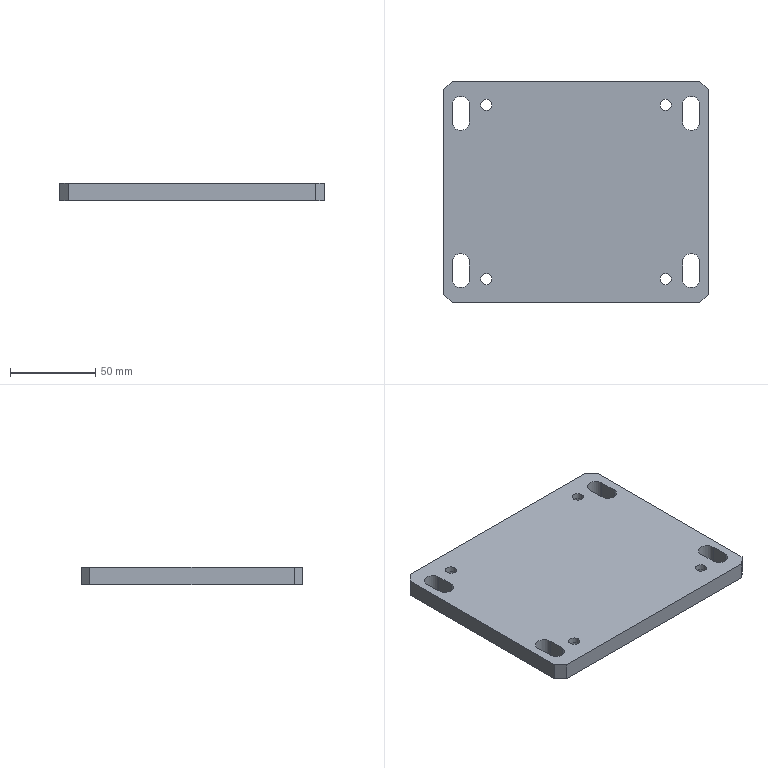Part | NX | 1 solid | 38 faces | box 155 x 130 x 10 mm | volume 190923 mm3 | plane 22 | cylinder 16 | commonest cylinder face diameters 10 x8 6.5 x4 11 x4
STEP:
#1=CARTESIAN_POINT('',(335.5,-45.,-18.));
#2=VERTEX_POINT('',#1);
#3=CARTESIAN_POINT('',(330.5,-40.,-18.));
#4=VERTEX_POINT('',#3);
#5=CARTESIAN_POINT('',(225.067,65.433,-18.));
#6=DIRECTION('',(-0.7071,0.7071,0.));
#7=VECTOR('',#6,1000.);
#8=LINE('',#5,#7);
#9=EDGE_CURVE('',#2,#4,#8,.T.);
#10=ORIENTED_EDGE('',*,*,#9,.F.);
#11=CARTESIAN_POINT('',(335.5,-45.,-28.));
#12=VERTEX_POINT('',#11);
#13=CARTESIAN_POINT('',(335.5,-45.,8.781));
#14=DIRECTION('',(0.,0.,1.));
#15=VECTOR('',#14,1000.);
#16=LINE('',#13,#15);
#17=EDGE_CURVE('',#12,#2,#16,.T.);
#18=ORIENTED_EDGE('',*,*,#17,.F.);
#19=CARTESIAN_POINT('',(330.5,-40.,-28.));
#20=VERTEX_POINT('',#19);
#21=CARTESIAN_POINT('',(407.933,-117.433,-28.));
#22=DIRECTION('',(0.7071,-0.7071,0.));
#23=VECTOR('',#22,1000.);
#24=LINE('',#21,#23);
#25=EDGE_CURVE('',#20,#12,#24,.T.);
#26=ORIENTED_EDGE('',*,*,#25,.F.);
#27=CARTESIAN_POINT('',(330.5,-40.,8.781));
#28=DIRECTION('',(0.,0.,-1.));
#29=VECTOR('',#28,1000.);
#30=LINE('',#27,#29);
#31=EDGE_CURVE('',#4,#20,#30,.T.);
#32=ORIENTED_EDGE('',*,*,#31,.F.);
#33=EDGE_LOOP('',(#10,#18,#26,#32));
#34=FACE_BOUND('',#33,.T.);
#35=CARTESIAN_POINT('',(335.5,-45.,8.781));
#36=DIRECTION('',(-0.7071,-0.7071,0.));
#37=DIRECTION('',(0.,0.,-1.));
#38=AXIS2_PLACEMENT_3D('',#35,#36,#37);
#39=PLANE('',#38);
#40=ADVANCED_FACE('',(#34),#39,.F.);
#41=CARTESIAN_POINT('',(316.,-156.,-28.));
#42=VERTEX_POINT('',#41);
#43=CARTESIAN_POINT('',(310.5,-156.,-28.));
#44=DIRECTION('',(0.,0.,1.));
#45=DIRECTION('',(1.,0.,0.));
#46=AXIS2_PLACEMENT_3D('',#43,#44,#45);
#47=CIRCLE('',#46,5.5);
#48=EDGE_CURVE('',#42,#42,#47,.T.);
#49=ORIENTED_EDGE('',*,*,#48,.F.);
#50=EDGE_LOOP('',(#49));
#51=FACE_BOUND('',#50,.T.);
#52=CARTESIAN_POINT('',(305.,-156.,-21.5));
#53=VERTEX_POINT('',#52);
#54=CARTESIAN_POINT('',(310.5,-156.,-21.5));
#55=DIRECTION('',(0.,0.,1.));
#56=DIRECTION('',(-1.,0.,0.));
#57=AXIS2_PLACEMENT_3D('',#54,#55,#56);
#58=CIRCLE('',#57,5.5);
#59=EDGE_CURVE('',#53,#53,#58,.T.);
#60=ORIENTED_EDGE('',*,*,#59,.T.);
#61=EDGE_LOOP('',(#60));
#62=FACE_BOUND('',#61,.T.);
#63=CARTESIAN_POINT('',(310.5,-156.,-28.));
#64=DIRECTION('',(0.,0.,1.));
#65=DIRECTION('',(0.,-1.,0.));
#66=AXIS2_PLACEMENT_3D('',#63,#64,#65);
#67=CYLINDRICAL_SURFACE('',#66,5.5);
#68=ADVANCED_FACE('',(#51,#62),#67,.F.);
#69=CARTESIAN_POINT('',(316.,-54.,-28.));
#70=VERTEX_POINT('',#69);
#71=CARTESIAN_POINT('',(310.5,-54.,-28.));
#72=DIRECTION('',(0.,0.,1.));
#73=DIRECTION('',(1.,0.,0.));
#74=AXIS2_PLACEMENT_3D('',#71,#72,#73);
#75=CIRCLE('',#74,5.5);
#76=EDGE_CURVE('',#70,#70,#75,.T.);
#77=ORIENTED_EDGE('',*,*,#76,.F.);
#78=EDGE_LOOP('',(#77));
#79=FACE_BOUND('',#78,.T.);
#80=CARTESIAN_POINT('',(316.,-54.,-21.5));
#81=VERTEX_POINT('',#80);
#82=CARTESIAN_POINT('',(310.5,-54.,-21.5));
#83=DIRECTION('',(0.,0.,1.));
#84=DIRECTION('',(1.,0.,0.));
#85=AXIS2_PLACEMENT_3D('',#82,#83,#84);
#86=CIRCLE('',#85,5.5);
#87=EDGE_CURVE('',#81,#81,#86,.T.);
#88=ORIENTED_EDGE('',*,*,#87,.T.);
#89=EDGE_LOOP('',(#88));
#90=FACE_BOUND('',#89,.T.);
#91=CARTESIAN_POINT('',(310.5,-54.,-28.));
#92=DIRECTION('',(0.,0.,1.));
#93=DIRECTION('',(0.,-1.,0.));
#94=AXIS2_PLACEMENT_3D('',#91,#92,#93);
#95=CYLINDRICAL_SURFACE('',#94,5.5);
#96=ADVANCED_FACE('',(#79,#90),#95,.F.);
#97=CARTESIAN_POINT('',(330.5,-54.,-18.));
#98=VERTEX_POINT('',#97);
#99=CARTESIAN_POINT('',(320.5,-54.,-18.));
#100=VERTEX_POINT('',#99);
#101=CARTESIAN_POINT('',(325.5,-54.,-18.));
#102=DIRECTION('',(0.,0.,1.));
#103=DIRECTION('',(1.,0.,0.));
#104=AXIS2_PLACEMENT_3D('',#101,#102,#103);
#105=CIRCLE('',#104,5.);
#106=EDGE_CURVE('',#98,#100,#105,.T.);
#107=ORIENTED_EDGE('',*,*,#106,.T.);
#108=CARTESIAN_POINT('',(320.5,-54.,-28.));
#109=VERTEX_POINT('',#108);
#110=CARTESIAN_POINT('',(320.5,-54.,-23.));
#111=DIRECTION('',(0.,0.,1.));
#112=VECTOR('',#111,1000.);
#113=LINE('',#110,#112);
#114=EDGE_CURVE('',#109,#100,#113,.T.);
#115=ORIENTED_EDGE('',*,*,#114,.F.);
#116=CARTESIAN_POINT('',(330.5,-54.,-28.));
#117=VERTEX_POINT('',#116);
#118=CARTESIAN_POINT('',(325.5,-54.,-28.));
#119=DIRECTION('',(0.,0.,-1.));
#120=DIRECTION('',(1.,0.,0.));
#121=AXIS2_PLACEMENT_3D('',#118,#119,#120);
#122=CIRCLE('',#121,5.);
#123=EDGE_CURVE('',#109,#117,#122,.T.);
#124=ORIENTED_EDGE('',*,*,#123,.T.);
#125=CARTESIAN_POINT('',(330.5,-54.,-23.));
#126=DIRECTION('',(0.,0.,-1.));
#127=VECTOR('',#126,1000.);
#128=LINE('',#125,#127);
#129=EDGE_CURVE('',#98,#117,#128,.T.);
#130=ORIENTED_EDGE('',*,*,#129,.F.);
#131=EDGE_LOOP('',(#107,#115,#124,#130));
#132=FACE_BOUND('',#131,.T.);
#133=CARTESIAN_POINT('',(325.5,-54.,-6.5));
#134=DIRECTION('',(0.,0.,-1.));
#135=DIRECTION('',(0.,1.,0.));
#136=AXIS2_PLACEMENT_3D('',#133,#134,#135);
#137=CYLINDRICAL_SURFACE('',#136,5.);
#138=ADVANCED_FACE('',(#132),#137,.F.);
#139=CARTESIAN_POINT('',(320.5,-64.,-18.));
#140=VERTEX_POINT('',#139);
#141=CARTESIAN_POINT('',(320.5,105.,-18.));
#142=DIRECTION('',(0.,-1.,0.));
#143=VECTOR('',#142,1000.);
#144=LINE('',#141,#143);
#145=EDGE_CURVE('',#100,#140,#144,.T.);
#146=ORIENTED_EDGE('',*,*,#145,.T.);
#147=CARTESIAN_POINT('',(320.5,-64.,-28.));
#148=VERTEX_POINT('',#147);
#149=CARTESIAN_POINT('',(320.5,-64.,-23.));
#150=DIRECTION('',(0.,0.,-1.));
#151=VECTOR('',#150,1000.);
#152=LINE('',#149,#151);
#153=EDGE_CURVE('',#140,#148,#152,.T.);
#154=ORIENTED_EDGE('',*,*,#153,.T.);
#155=CARTESIAN_POINT('',(320.5,105.,-28.));
#156=DIRECTION('',(0.,1.,0.));
#157=VECTOR('',#156,1000.);
#158=LINE('',#155,#157);
#159=EDGE_CURVE('',#148,#109,#158,.T.);
#160=ORIENTED_EDGE('',*,*,#159,.T.);
#161=ORIENTED_EDGE('',*,*,#114,.T.);
#162=EDGE_LOOP('',(#146,#154,#160,#161));
#163=FACE_BOUND('',#162,.T.);
#164=CARTESIAN_POINT('',(320.5,-53.,-6.5));
#165=DIRECTION('',(-1.,0.,0.));
#166=DIRECTION('',(0.,0.,-1.));
#167=AXIS2_PLACEMENT_3D('',#164,#165,#166);
#168=PLANE('',#167);
#169=ADVANCED_FACE('',(#163),#168,.F.);
#170=CARTESIAN_POINT('',(330.5,-64.,-18.));
#171=VERTEX_POINT('',#170);
#172=CARTESIAN_POINT('',(325.5,-64.,-18.));
#173=DIRECTION('',(0.,0.,1.));
#174=DIRECTION('',(1.,0.,0.));
#175=AXIS2_PLACEMENT_3D('',#172,#173,#174);
#176=CIRCLE('',#175,5.);
#177=EDGE_CURVE('',#140,#171,#176,.T.);
#178=ORIENTED_EDGE('',*,*,#177,.T.);
#179=CARTESIAN_POINT('',(330.5,-64.,-28.));
#180=VERTEX_POINT('',#179);
#181=CARTESIAN_POINT('',(330.5,-64.,-23.));
#182=DIRECTION('',(0.,0.,1.));
#183=VECTOR('',#182,1000.);
#184=LINE('',#181,#183);
#185=EDGE_CURVE('',#180,#171,#184,.T.);
#186=ORIENTED_EDGE('',*,*,#185,.F.);
#187=CARTESIAN_POINT('',(325.5,-64.,-28.));
#188=DIRECTION('',(0.,0.,-1.));
#189=DIRECTION('',(1.,0.,0.));
#190=AXIS2_PLACEMENT_3D('',#187,#188,#189);
#191=CIRCLE('',#190,5.);
#192=EDGE_CURVE('',#180,#148,#191,.T.);
#193=ORIENTED_EDGE('',*,*,#192,.T.);
#194=ORIENTED_EDGE('',*,*,#153,.F.);
#195=EDGE_LOOP('',(#178,#186,#193,#194));
#196=FACE_BOUND('',#195,.T.);
#197=CARTESIAN_POINT('',(325.5,-64.,-6.5));
#198=DIRECTION('',(0.,0.,-1.));
#199=DIRECTION('',(0.,1.,0.));
#200=AXIS2_PLACEMENT_3D('',#197,#198,#199);
#201=CYLINDRICAL_SURFACE('',#200,5.);
#202=ADVANCED_FACE('',(#196),#201,.F.);
#203=CARTESIAN_POINT('',(330.5,105.,-18.));
#204=DIRECTION('',(0.,1.,0.));
#205=VECTOR('',#204,1000.);
#206=LINE('',#203,#205);
#207=EDGE_CURVE('',#171,#98,#206,.T.);
#208=ORIENTED_EDGE('',*,*,#207,.T.);
#209=ORIENTED_EDGE('',*,*,#129,.T.);
#210=CARTESIAN_POINT('',(330.5,105.,-28.));
#211=DIRECTION('',(0.,-1.,0.));
#212=VECTOR('',#211,1000.);
#213=LINE('',#210,#212);
#214=EDGE_CURVE('',#117,#180,#213,.T.);
#215=ORIENTED_EDGE('',*,*,#214,.T.);
#216=ORIENTED_EDGE('',*,*,#185,.T.);
#217=EDGE_LOOP('',(#208,#209,#215,#216));
#218=FACE_BOUND('',#217,.T.);
#219=CARTESIAN_POINT('',(330.5,-53.,-6.5));
#220=DIRECTION('',(1.,0.,0.));
#221=DIRECTION('',(0.,0.,1.));
#222=AXIS2_PLACEMENT_3D('',#219,#220,#221);
#223=PLANE('',#222);
#224=ADVANCED_FACE('',(#218),#223,.F.);
#225=CARTESIAN_POINT('',(320.5,-156.,-18.));
#226=VERTEX_POINT('',#225);
#227=CARTESIAN_POINT('',(330.5,-156.,-18.));
#228=VERTEX_POINT('',#227);
#229=CARTESIAN_POINT('',(325.5,-156.,-18.));
#230=DIRECTION('',(0.,0.,1.));
#231=DIRECTION('',(1.,0.,0.));
#232=AXIS2_PLACEMENT_3D('',#229,#230,#231);
#233=CIRCLE('',#232,5.);
#234=EDGE_CURVE('',#226,#228,#233,.T.);
#235=ORIENTED_EDGE('',*,*,#234,.T.);
#236=CARTESIAN_POINT('',(330.5,-156.,-28.));
#237=VERTEX_POINT('',#236);
#238=CARTESIAN_POINT('',(330.5,-156.,-6.5));
#239=DIRECTION('',(0.,0.,1.));
#240=VECTOR('',#239,1000.);
#241=LINE('',#238,#240);
#242=EDGE_CURVE('',#237,#228,#241,.T.);
#243=ORIENTED_EDGE('',*,*,#242,.F.);
#244=CARTESIAN_POINT('',(320.5,-156.,-28.));
#245=VERTEX_POINT('',#244);
#246=CARTESIAN_POINT('',(325.5,-156.,-28.));
#247=DIRECTION('',(0.,0.,-1.));
#248=DIRECTION('',(1.,0.,0.));
#249=AXIS2_PLACEMENT_3D('',#246,#247,#248);
#250=CIRCLE('',#249,5.);
#251=EDGE_CURVE('',#237,#245,#250,.T.);
#252=ORIENTED_EDGE('',*,*,#251,.T.);
#253=CARTESIAN_POINT('',(320.5,-156.,-6.5));
#254=DIRECTION('',(0.,0.,-1.));
#255=VECTOR('',#254,1000.);
#256=LINE('',#253,#255);
#257=EDGE_CURVE('',#226,#245,#256,.T.);
#258=ORIENTED_EDGE('',*,*,#257,.F.);
#259=EDGE_LOOP('',(#235,#243,#252,#258));
#260=FACE_BOUND('',#259,.T.);
#261=CARTESIAN_POINT('',(325.5,-156.,-6.5));
#262=DIRECTION('',(0.,0.,-1.));
#263=DIRECTION('',(0.,-1.,0.));
#264=AXIS2_PLACEMENT_3D('',#261,#262,#263);
#265=CYLINDRICAL_SURFACE('',#264,5.);
#266=ADVANCED_FACE('',(#260),#265,.F.);
#267=CARTESIAN_POINT('',(330.5,-146.,-18.));
#268=VERTEX_POINT('',#267);
#269=CARTESIAN_POINT('',(330.5,-53.,-18.));
#270=DIRECTION('',(0.,1.,0.));
#271=VECTOR('',#270,1000.);
#272=LINE('',#269,#271);
#273=EDGE_CURVE('',#228,#268,#272,.T.);
#274=ORIENTED_EDGE('',*,*,#273,.T.);
#275=CARTESIAN_POINT('',(330.5,-146.,-28.));
#276=VERTEX_POINT('',#275);
#277=CARTESIAN_POINT('',(330.5,-146.,-6.5));
#278=DIRECTION('',(0.,0.,-1.));
#279=VECTOR('',#278,1000.);
#280=LINE('',#277,#279);
#281=EDGE_CURVE('',#268,#276,#280,.T.);
#282=ORIENTED_EDGE('',*,*,#281,.T.);
#283=CARTESIAN_POINT('',(330.5,-53.,-28.));
#284=DIRECTION('',(0.,-1.,0.));
#285=VECTOR('',#284,1000.);
#286=LINE('',#283,#285);
#287=EDGE_CURVE('',#276,#237,#286,.T.);
#288=ORIENTED_EDGE('',*,*,#287,.T.);
#289=ORIENTED_EDGE('',*,*,#242,.T.);
#290=EDGE_LOOP('',(#274,#282,#288,#289));
#291=FACE_BOUND('',#290,.T.);
#292=CARTESIAN_POINT('',(330.5,-53.,-6.5));
#293=DIRECTION('',(1.,0.,0.));
#294=DIRECTION('',(0.,0.,1.));
#295=AXIS2_PLACEMENT_3D('',#292,#293,#294);
#296=PLANE('',#295);
#297=ADVANCED_FACE('',(#291),#296,.F.);
#298=CARTESIAN_POINT('',(320.5,-146.,-18.));
#299=VERTEX_POINT('',#298);
#300=CARTESIAN_POINT('',(325.5,-146.,-18.));
#301=DIRECTION('',(0.,0.,1.));
#302=DIRECTION('',(1.,0.,0.));
#303=AXIS2_PLACEMENT_3D('',#300,#301,#302);
#304=CIRCLE('',#303,5.);
#305=EDGE_CURVE('',#268,#299,#304,.T.);
#306=ORIENTED_EDGE('',*,*,#305,.T.);
#307=CARTESIAN_POINT('',(320.5,-146.,-28.));
#308=VERTEX_POINT('',#307);
#309=CARTESIAN_POINT('',(320.5,-146.,-6.5));
#310=DIRECTION('',(0.,0.,1.));
#311=VECTOR('',#310,1000.);
#312=LINE('',#309,#311);
#313=EDGE_CURVE('',#308,#299,#312,.T.);
#314=ORIENTED_EDGE('',*,*,#313,.F.);
#315=CARTESIAN_POINT('',(325.5,-146.,-28.));
#316=DIRECTION('',(0.,0.,-1.));
#317=DIRECTION('',(1.,0.,0.));
#318=AXIS2_PLACEMENT_3D('',#315,#316,#317);
#319=CIRCLE('',#318,5.);
#320=EDGE_CURVE('',#308,#276,#319,.T.);
#321=ORIENTED_EDGE('',*,*,#320,.T.);
#322=ORIENTED_EDGE('',*,*,#281,.F.);
#323=EDGE_LOOP('',(#306,#314,#321,#322));
#324=FACE_BOUND('',#323,.T.);
#325=CARTESIAN_POINT('',(325.5,-146.,-6.5));
#326=DIRECTION('',(0.,0.,-1.));
#327=DIRECTION('',(0.,-1.,0.));
#328=AXIS2_PLACEMENT_3D('',#325,#326,#327);
#329=CYLINDRICAL_SURFACE('',#328,5.);
#330=ADVANCED_FACE('',(#324),#329,.F.);
#331=CARTESIAN_POINT('',(320.5,-53.,-18.));
#332=DIRECTION('',(0.,-1.,0.));
#333=VECTOR('',#332,1000.);
#334=LINE('',#331,#333);
#335=EDGE_CURVE('',#299,#226,#334,.T.);
#336=ORIENTED_EDGE('',*,*,#335,.T.);
#337=ORIENTED_EDGE('',*,*,#257,.T.);
#338=CARTESIAN_POINT('',(320.5,-53.,-28.));
#339=DIRECTION('',(0.,1.,0.));
#340=VECTOR('',#339,1000.);
#341=LINE('',#338,#340);
#342=EDGE_CURVE('',#245,#308,#341,.T.);
#343=ORIENTED_EDGE('',*,*,#342,.T.);
#344=ORIENTED_EDGE('',*,*,#313,.T.);
#345=EDGE_LOOP('',(#336,#337,#343,#344));
#346=FACE_BOUND('',#345,.T.);
#347=CARTESIAN_POINT('',(320.5,-53.,-6.5));
#348=DIRECTION('',(-1.,0.,0.));
#349=DIRECTION('',(0.,0.,-1.));
#350=AXIS2_PLACEMENT_3D('',#347,#348,#349);
#351=PLANE('',#350);
#352=ADVANCED_FACE('',(#346),#351,.F.);
#353=CARTESIAN_POINT('',(335.5,-165.,-28.));
#354=VERTEX_POINT('',#353);
#355=CARTESIAN_POINT('',(335.5,-315.,-28.));
#356=DIRECTION('',(0.,-1.,0.));
#357=VECTOR('',#356,1000.);
#358=LINE('',#355,#357);
#359=EDGE_CURVE('',#12,#354,#358,.T.);
#360=ORIENTED_EDGE('',*,*,#359,.F.);
#361=ORIENTED_EDGE('',*,*,#17,.T.);
#362=CARTESIAN_POINT('',(335.5,-165.,-18.));
#363=VERTEX_POINT('',#362);
#364=CARTESIAN_POINT('',(335.5,105.,-18.));
#365=DIRECTION('',(0.,1.,0.));
#366=VECTOR('',#365,1000.);
#367=LINE('',#364,#366);
#368=EDGE_CURVE('',#363,#2,#367,.T.);
#369=ORIENTED_EDGE('',*,*,#368,.F.);
#370=CARTESIAN_POINT('',(335.5,-165.,8.781));
#371=DIRECTION('',(0.,0.,-1.));
#372=VECTOR('',#371,1000.);
#373=LINE('',#370,#372);
#374=EDGE_CURVE('',#363,#354,#373,.T.);
#375=ORIENTED_EDGE('',*,*,#374,.T.);
#376=EDGE_LOOP('',(#360,#361,#369,#375));
#377=FACE_BOUND('',#376,.T.);
#378=CARTESIAN_POINT('',(335.5,-105.,8.781));
#379=DIRECTION('',(1.,0.,0.));
#380=DIRECTION('',(0.,0.,-1.));
#381=AXIS2_PLACEMENT_3D('',#378,#379,#380);
#382=PLANE('',#381);
#383=ADVANCED_FACE('',(#377),#382,.T.);
#384=CARTESIAN_POINT('',(330.5,-170.,-28.));
#385=VERTEX_POINT('',#384);
#386=CARTESIAN_POINT('',(197.933,-302.567,-28.));
#387=DIRECTION('',(-0.7071,-0.7071,0.));
#388=VECTOR('',#387,1000.);
#389=LINE('',#386,#388);
#390=EDGE_CURVE('',#354,#385,#389,.T.);
#391=ORIENTED_EDGE('',*,*,#390,.F.);
#392=ORIENTED_EDGE('',*,*,#374,.F.);
#393=CARTESIAN_POINT('',(330.5,-170.,-18.));
#394=VERTEX_POINT('',#393);
#395=CARTESIAN_POINT('',(435.067,-65.433,-18.));
#396=DIRECTION('',(0.7071,0.7071,0.));
#397=VECTOR('',#396,1000.);
#398=LINE('',#395,#397);
#399=EDGE_CURVE('',#394,#363,#398,.T.);
#400=ORIENTED_EDGE('',*,*,#399,.F.);
#401=CARTESIAN_POINT('',(330.5,-170.,8.781));
#402=DIRECTION('',(0.,0.,1.));
#403=VECTOR('',#402,1000.);
#404=LINE('',#401,#403);
#405=EDGE_CURVE('',#385,#394,#404,.T.);
#406=ORIENTED_EDGE('',*,*,#405,.F.);
#407=EDGE_LOOP('',(#391,#392,#400,#406));
#408=FACE_BOUND('',#407,.T.);
#409=CARTESIAN_POINT('',(335.5,-165.,8.781));
#410=DIRECTION('',(-0.7071,0.7071,0.));
#411=DIRECTION('',(0.,0.,1.));
#412=AXIS2_PLACEMENT_3D('',#409,#410,#411);
#413=PLANE('',#412);
#414=ADVANCED_FACE('',(#408),#413,.F.);
#415=CARTESIAN_POINT('',(313.75,-54.,-18.));
#416=VERTEX_POINT('',#415);
#417=CARTESIAN_POINT('',(310.5,-54.,-18.));
#418=DIRECTION('',(0.,0.,-1.));
#419=DIRECTION('',(1.,0.,0.));
#420=AXIS2_PLACEMENT_3D('',#417,#418,#419);
#421=CIRCLE('',#420,3.25);
#422=EDGE_CURVE('',#416,#416,#421,.T.);
#423=ORIENTED_EDGE('',*,*,#422,.F.);
#424=EDGE_LOOP('',(#423));
#425=FACE_BOUND('',#424,.T.);
#426=CARTESIAN_POINT('',(313.75,-54.,-21.5));
#427=VERTEX_POINT('',#426);
#428=CARTESIAN_POINT('',(310.5,-54.,-21.5));
#429=DIRECTION('',(0.,0.,1.));
#430=DIRECTION('',(1.,0.,0.));
#431=AXIS2_PLACEMENT_3D('',#428,#429,#430);
#432=CIRCLE('',#431,3.25);
#433=EDGE_CURVE('',#427,#427,#432,.T.);
#434=ORIENTED_EDGE('',*,*,#433,.F.);
#435=EDGE_LOOP('',(#434));
#436=FACE_BOUND('',#435,.T.);
#437=CARTESIAN_POINT('',(310.5,-54.,-108.));
#438=DIRECTION('',(0.,0.,1.));
#439=DIRECTION('',(0.,1.,0.));
#440=AXIS2_PLACEMENT_3D('',#437,#438,#439);
#441=CYLINDRICAL_SURFACE('',#440,3.25);
#442=ADVANCED_FACE('',(#425,#436),#441,.F.);
#443=CARTESIAN_POINT('',(313.75,-156.,-18.));
#444=VERTEX_POINT('',#443);
#445=CARTESIAN_POINT('',(310.5,-156.,-18.));
#446=DIRECTION('',(0.,0.,-1.));
#447=DIRECTION('',(1.,0.,0.));
#448=AXIS2_PLACEMENT_3D('',#445,#446,#447);
#449=CIRCLE('',#448,3.25);
#450=EDGE_CURVE('',#444,#444,#449,.T.);
#451=ORIENTED_EDGE('',*,*,#450,.F.);
#452=EDGE_LOOP('',(#451));
#453=FACE_BOUND('',#452,.T.);
#454=CARTESIAN_POINT('',(307.25,-156.,-21.5));
#455=VERTEX_POINT('',#454);
#456=CARTESIAN_POINT('',(310.5,-156.,-21.5));
#457=DIRECTION('',(0.,0.,1.));
#458=DIRECTION('',(-1.,0.,0.));
#459=AXIS2_PLACEMENT_3D('',#456,#457,#458);
#460=CIRCLE('',#459,3.25);
#461=EDGE_CURVE('',#455,#455,#460,.T.);
#462=ORIENTED_EDGE('',*,*,#461,.F.);
#463=EDGE_LOOP('',(#462));
#464=FACE_BOUND('',#463,.T.);
#465=CARTESIAN_POINT('',(310.5,-156.,-108.));
#466=DIRECTION('',(0.,0.,1.));
#467=DIRECTION('',(0.,1.,0.));
#468=AXIS2_PLACEMENT_3D('',#465,#466,#467);
#469=CYLINDRICAL_SURFACE('',#468,3.25);
#470=ADVANCED_FACE('',(#453,#464),#469,.F.);
#471=ORIENTED_EDGE('',*,*,#59,.F.);
#472=EDGE_LOOP('',(#471));
#473=FACE_BOUND('',#472,.T.);
#474=ORIENTED_EDGE('',*,*,#461,.T.);
#475=EDGE_LOOP('',(#474));
#476=FACE_BOUND('',#475,.T.);
#477=CARTESIAN_POINT('',(310.5,-156.,-21.5));
#478=DIRECTION('',(0.,0.,1.));
#479=DIRECTION('',(0.,1.,0.));
#480=AXIS2_PLACEMENT_3D('',#477,#478,#479);
#481=PLANE('',#480);
#482=ADVANCED_FACE('',(#473,#476),#481,.F.);
#483=ORIENTED_EDGE('',*,*,#87,.F.);
#484=EDGE_LOOP('',(#483));
#485=FACE_BOUND('',#484,.T.);
#486=ORIENTED_EDGE('',*,*,#433,.T.);
#487=EDGE_LOOP('',(#486));
#488=FACE_BOUND('',#487,.T.);
#489=CARTESIAN_POINT('',(310.5,-156.,-21.5));
#490=DIRECTION('',(0.,0.,1.));
#491=DIRECTION('',(0.,1.,0.));
#492=AXIS2_PLACEMENT_3D('',#489,#490,#491);
#493=PLANE('',#492);
#494=ADVANCED_FACE('',(#485,#488),#493,.F.);
#495=ORIENTED_EDGE('',*,*,#234,.F.);
#496=ORIENTED_EDGE('',*,*,#335,.F.);
#497=ORIENTED_EDGE('',*,*,#305,.F.);
#498=ORIENTED_EDGE('',*,*,#273,.F.);
#499=EDGE_LOOP('',(#495,#496,#497,#498));
#500=FACE_BOUND('',#499,.T.);
#501=ORIENTED_EDGE('',*,*,#106,.F.);
#502=ORIENTED_EDGE('',*,*,#207,.F.);
#503=ORIENTED_EDGE('',*,*,#177,.F.);
#504=ORIENTED_EDGE('',*,*,#145,.F.);
#505=EDGE_LOOP('',(#501,#502,#503,#504));
#506=FACE_BOUND('',#505,.T.);
#507=ORIENTED_EDGE('',*,*,#450,.T.);
#508=EDGE_LOOP('',(#507));
#509=FACE_BOUND('',#508,.T.);
#510=ORIENTED_EDGE('',*,*,#422,.T.);
#511=EDGE_LOOP('',(#510));
#512=FACE_BOUND('',#511,.T.);
#513=CARTESIAN_POINT('',(185.5,-170.,-18.));
#514=VERTEX_POINT('',#513);
#515=CARTESIAN_POINT('',(274.635,-170.,-18.));
#516=DIRECTION('',(1.,0.,0.));
#517=VECTOR('',#516,1000.);
#518=LINE('',#515,#517);
#519=EDGE_CURVE('',#514,#394,#518,.T.);
#520=ORIENTED_EDGE('',*,*,#519,.T.);
#521=ORIENTED_EDGE('',*,*,#399,.T.);
#522=ORIENTED_EDGE('',*,*,#368,.T.);
#523=ORIENTED_EDGE('',*,*,#9,.T.);
#524=CARTESIAN_POINT('',(185.5,-40.,-18.));
#525=VERTEX_POINT('',#524);
#526=CARTESIAN_POINT('',(276.1,-40.,-18.));
#527=DIRECTION('',(1.,0.,0.));
#528=VECTOR('',#527,1000.);
#529=LINE('',#526,#528);
#530=EDGE_CURVE('',#525,#4,#529,.T.);
#531=ORIENTED_EDGE('',*,*,#530,.F.);
#532=CARTESIAN_POINT('',(180.5,-45.,-18.));
#533=VERTEX_POINT('',#532);
#534=CARTESIAN_POINT('',(307.567,82.067,-18.));
#535=DIRECTION('',(-0.7071,-0.7071,0.));
#536=VECTOR('',#535,1000.);
#537=LINE('',#534,#536);
#538=EDGE_CURVE('',#525,#533,#537,.T.);
#539=ORIENTED_EDGE('',*,*,#538,.T.);
#540=CARTESIAN_POINT('',(180.5,-165.,-18.));
#541=VERTEX_POINT('',#540);
#542=CARTESIAN_POINT('',(180.5,105.,-18.));
#543=DIRECTION('',(0.,-1.,0.));
#544=VECTOR('',#543,1000.);
#545=LINE('',#542,#544);
#546=EDGE_CURVE('',#533,#541,#545,.T.);
#547=ORIENTED_EDGE('',*,*,#546,.T.);
#548=CARTESIAN_POINT('',(97.567,-82.067,-18.));
#549=DIRECTION('',(0.7071,-0.7071,0.));
#550=VECTOR('',#549,1000.);
#551=LINE('',#548,#550);
#552=EDGE_CURVE('',#541,#514,#551,.T.);
#553=ORIENTED_EDGE('',*,*,#552,.T.);
#554=EDGE_LOOP('',(#520,#521,#522,#523,#531,#539,#547,#553));
#555=FACE_BOUND('',#554,.T.);
#556=CARTESIAN_POINT('',(195.5,-54.,-18.));
#557=VERTEX_POINT('',#556);
#558=CARTESIAN_POINT('',(185.5,-54.,-18.));
#559=VERTEX_POINT('',#558);
#560=CARTESIAN_POINT('',(190.5,-54.,-18.));
#561=DIRECTION('',(0.,0.,1.));
#562=DIRECTION('',(1.,0.,0.));
#563=AXIS2_PLACEMENT_3D('',#560,#561,#562);
#564=CIRCLE('',#563,5.);
#565=EDGE_CURVE('',#557,#559,#564,.T.);
#566=ORIENTED_EDGE('',*,*,#565,.F.);
#567=CARTESIAN_POINT('',(195.5,-64.,-18.));
#568=VERTEX_POINT('',#567);
#569=CARTESIAN_POINT('',(195.5,-157.,-18.));
#570=DIRECTION('',(0.,1.,0.));
#571=VECTOR('',#570,1000.);
#572=LINE('',#569,#571);
#573=EDGE_CURVE('',#568,#557,#572,.T.);
#574=ORIENTED_EDGE('',*,*,#573,.F.);
#575=CARTESIAN_POINT('',(185.5,-64.,-18.));
#576=VERTEX_POINT('',#575);
#577=CARTESIAN_POINT('',(190.5,-64.,-18.));
#578=DIRECTION('',(0.,0.,1.));
#579=DIRECTION('',(1.,0.,0.));
#580=AXIS2_PLACEMENT_3D('',#577,#578,#579);
#581=CIRCLE('',#580,5.);
#582=EDGE_CURVE('',#576,#568,#581,.T.);
#583=ORIENTED_EDGE('',*,*,#582,.F.);
#584=CARTESIAN_POINT('',(185.5,-157.,-18.));
#585=DIRECTION('',(0.,-1.,0.));
#586=VECTOR('',#585,1000.);
#587=LINE('',#584,#586);
#588=EDGE_CURVE('',#559,#576,#587,.T.);
#589=ORIENTED_EDGE('',*,*,#588,.F.);
#590=EDGE_LOOP('',(#566,#574,#583,#589));
#591=FACE_BOUND('',#590,.T.);
#592=CARTESIAN_POINT('',(185.5,-156.,-18.));
#593=VERTEX_POINT('',#592);
#594=CARTESIAN_POINT('',(195.5,-156.,-18.));
#595=VERTEX_POINT('',#594);
#596=CARTESIAN_POINT('',(190.5,-156.,-18.));
#597=DIRECTION('',(0.,0.,1.));
#598=DIRECTION('',(1.,0.,0.));
#599=AXIS2_PLACEMENT_3D('',#596,#597,#598);
#600=CIRCLE('',#599,5.);
#601=EDGE_CURVE('',#593,#595,#600,.T.);
#602=ORIENTED_EDGE('',*,*,#601,.F.);
#603=CARTESIAN_POINT('',(185.5,-146.,-18.));
#604=VERTEX_POINT('',#603);
#605=CARTESIAN_POINT('',(185.5,105.,-18.));
#606=DIRECTION('',(0.,-1.,0.));
#607=VECTOR('',#606,1000.);
#608=LINE('',#605,#607);
#609=EDGE_CURVE('',#604,#593,#608,.T.);
#610=ORIENTED_EDGE('',*,*,#609,.F.);
#611=CARTESIAN_POINT('',(195.5,-146.,-18.));
#612=VERTEX_POINT('',#611);
#613=CARTESIAN_POINT('',(190.5,-146.,-18.));
#614=DIRECTION('',(0.,0.,1.));
#615=DIRECTION('',(1.,0.,0.));
#616=AXIS2_PLACEMENT_3D('',#613,#614,#615);
#617=CIRCLE('',#616,5.);
#618=EDGE_CURVE('',#612,#604,#617,.T.);
#619=ORIENTED_EDGE('',*,*,#618,.F.);
#620=CARTESIAN_POINT('',(195.5,105.,-18.));
#621=DIRECTION('',(0.,1.,0.));
#622=VECTOR('',#621,1000.);
#623=LINE('',#620,#622);
#624=EDGE_CURVE('',#595,#612,#623,.T.);
#625=ORIENTED_EDGE('',*,*,#624,.F.);
#626=EDGE_LOOP('',(#602,#610,#619,#625));
#627=FACE_BOUND('',#626,.T.);
#628=CARTESIAN_POINT('',(208.75,-54.,-18.));
#629=VERTEX_POINT('',#628);
#630=CARTESIAN_POINT('',(205.5,-54.,-18.));
#631=DIRECTION('',(0.,0.,-1.));
#632=DIRECTION('',(1.,0.,0.));
#633=AXIS2_PLACEMENT_3D('',#630,#631,#632);
#634=CIRCLE('',#633,3.25);
#635=EDGE_CURVE('',#629,#629,#634,.T.);
#636=ORIENTED_EDGE('',*,*,#635,.T.);
#637=EDGE_LOOP('',(#636));
#638=FACE_BOUND('',#637,.T.);
#639=CARTESIAN_POINT('',(208.75,-156.,-18.));
#640=VERTEX_POINT('',#639);
#641=CARTESIAN_POINT('',(205.5,-156.,-18.));
#642=DIRECTION('',(0.,0.,-1.));
#643=DIRECTION('',(1.,0.,0.));
#644=AXIS2_PLACEMENT_3D('',#641,#642,#643);
#645=CIRCLE('',#644,3.25);
#646=EDGE_CURVE('',#640,#640,#645,.T.);
#647=ORIENTED_EDGE('',*,*,#646,.T.);
#648=EDGE_LOOP('',(#647));
#649=FACE_BOUND('',#648,.T.);
#650=CARTESIAN_POINT('',(274.635,105.,-18.));
#651=DIRECTION('',(0.,0.,-1.));
#652=DIRECTION('',(0.,1.,0.));
#653=AXIS2_PLACEMENT_3D('',#650,#651,#652);
#654=PLANE('',#653);
#655=ADVANCED_FACE('',(#500,#506,#509,#512,#555,#591,#627,#638,#649),#654,.F.);
#656=ORIENTED_EDGE('',*,*,#530,.T.);
#657=ORIENTED_EDGE('',*,*,#31,.T.);
#658=CARTESIAN_POINT('',(185.5,-40.,-28.));
#659=VERTEX_POINT('',#658);
#660=CARTESIAN_POINT('',(274.635,-40.,-28.));
#661=DIRECTION('',(1.,0.,0.));
#662=VECTOR('',#661,1000.);
#663=LINE('',#660,#662);
#664=EDGE_CURVE('',#659,#20,#663,.T.);
#665=ORIENTED_EDGE('',*,*,#664,.F.);
#666=CARTESIAN_POINT('',(185.5,-40.,8.781));
#667=DIRECTION('',(0.,0.,1.));
#668=VECTOR('',#667,1000.);
#669=LINE('',#666,#668);
#670=EDGE_CURVE('',#659,#525,#669,.T.);
#671=ORIENTED_EDGE('',*,*,#670,.T.);
#672=EDGE_LOOP('',(#656,#657,#665,#671));
#673=FACE_BOUND('',#672,.T.);
#674=CARTESIAN_POINT('',(276.1,-40.,8.781));
#675=DIRECTION('',(0.,1.,0.));
#676=DIRECTION('',(0.,0.,1.));
#677=AXIS2_PLACEMENT_3D('',#674,#675,#676);
#678=PLANE('',#677);
#679=ADVANCED_FACE('',(#673),#678,.T.);
#680=ORIENTED_EDGE('',*,*,#251,.F.);
#681=ORIENTED_EDGE('',*,*,#287,.F.);
#682=ORIENTED_EDGE('',*,*,#320,.F.);
#683=ORIENTED_EDGE('',*,*,#342,.F.);
#684=EDGE_LOOP('',(#680,#681,#682,#683));
#685=FACE_BOUND('',#684,.T.);
#686=ORIENTED_EDGE('',*,*,#123,.F.);
#687=ORIENTED_EDGE('',*,*,#159,.F.);
#688=ORIENTED_EDGE('',*,*,#192,.F.);
#689=ORIENTED_EDGE('',*,*,#214,.F.);
#690=EDGE_LOOP('',(#686,#687,#688,#689));
#691=FACE_BOUND('',#690,.T.);
#692=ORIENTED_EDGE('',*,*,#76,.T.);
#693=EDGE_LOOP('',(#692));
#694=FACE_BOUND('',#693,.T.);
#695=ORIENTED_EDGE('',*,*,#48,.T.);
#696=EDGE_LOOP('',(#695));
#697=FACE_BOUND('',#696,.T.);
#698=ORIENTED_EDGE('',*,*,#664,.T.);
#699=ORIENTED_EDGE('',*,*,#25,.T.);
#700=ORIENTED_EDGE('',*,*,#359,.T.);
#701=ORIENTED_EDGE('',*,*,#390,.T.);
#702=CARTESIAN_POINT('',(185.5,-170.,-28.));
#703=VERTEX_POINT('',#702);
#704=CARTESIAN_POINT('',(276.1,-170.,-28.));
#705=DIRECTION('',(1.,0.,0.));
#706=VECTOR('',#705,1000.);
#707=LINE('',#704,#706);
#708=EDGE_CURVE('',#703,#385,#707,.T.);
#709=ORIENTED_EDGE('',*,*,#708,.F.);
#710=CARTESIAN_POINT('',(180.5,-165.,-28.));
#711=VERTEX_POINT('',#710);
#712=CARTESIAN_POINT('',(108.067,-92.567,-28.));
#713=DIRECTION('',(-0.7071,0.7071,0.));
#714=VECTOR('',#713,1000.);
#715=LINE('',#712,#714);
#716=EDGE_CURVE('',#703,#711,#715,.T.);
#717=ORIENTED_EDGE('',*,*,#716,.T.);
#718=CARTESIAN_POINT('',(180.5,-45.,-28.));
#719=VERTEX_POINT('',#718);
#720=CARTESIAN_POINT('',(180.5,105.,-28.));
#721=DIRECTION('',(0.,1.,0.));
#722=VECTOR('',#721,1000.);
#723=LINE('',#720,#722);
#724=EDGE_CURVE('',#711,#719,#723,.T.);
#725=ORIENTED_EDGE('',*,*,#724,.T.);
#726=CARTESIAN_POINT('',(318.067,92.567,-28.));
#727=DIRECTION('',(0.7071,0.7071,0.));
#728=VECTOR('',#727,1000.);
#729=LINE('',#726,#728);
#730=EDGE_CURVE('',#719,#659,#729,.T.);
#731=ORIENTED_EDGE('',*,*,#730,.T.);
#732=EDGE_LOOP('',(#698,#699,#700,#701,#709,#717,#725,#731));
#733=FACE_BOUND('',#732,.T.);
#734=CARTESIAN_POINT('',(185.5,-54.,-28.));
#735=VERTEX_POINT('',#734);
#736=CARTESIAN_POINT('',(195.5,-54.,-28.));
#737=VERTEX_POINT('',#736);
#738=CARTESIAN_POINT('',(190.5,-54.,-28.));
#739=DIRECTION('',(0.,0.,-1.));
#740=DIRECTION('',(1.,0.,0.));
#741=AXIS2_PLACEMENT_3D('',#738,#739,#740);
#742=CIRCLE('',#741,5.);
#743=EDGE_CURVE('',#735,#737,#742,.T.);
#744=ORIENTED_EDGE('',*,*,#743,.F.);
#745=CARTESIAN_POINT('',(185.5,-64.,-28.));
#746=VERTEX_POINT('',#745);
#747=CARTESIAN_POINT('',(185.5,-157.,-28.));
#748=DIRECTION('',(0.,1.,0.));
#749=VECTOR('',#748,1000.);
#750=LINE('',#747,#749);
#751=EDGE_CURVE('',#746,#735,#750,.T.);
#752=ORIENTED_EDGE('',*,*,#751,.F.);
#753=CARTESIAN_POINT('',(195.5,-64.,-28.));
#754=VERTEX_POINT('',#753);
#755=CARTESIAN_POINT('',(190.5,-64.,-28.));
#756=DIRECTION('',(0.,0.,-1.));
#757=DIRECTION('',(1.,0.,0.));
#758=AXIS2_PLACEMENT_3D('',#755,#756,#757);
#759=CIRCLE('',#758,5.);
#760=EDGE_CURVE('',#754,#746,#759,.T.);
#761=ORIENTED_EDGE('',*,*,#760,.F.);
#762=CARTESIAN_POINT('',(195.5,-157.,-28.));
#763=DIRECTION('',(0.,-1.,0.));
#764=VECTOR('',#763,1000.);
#765=LINE('',#762,#764);
#766=EDGE_CURVE('',#737,#754,#765,.T.);
#767=ORIENTED_EDGE('',*,*,#766,.F.);
#768=EDGE_LOOP('',(#744,#752,#761,#767));
#769=FACE_BOUND('',#768,.T.);
#770=CARTESIAN_POINT('',(195.5,-156.,-28.));
#771=VERTEX_POINT('',#770);
#772=CARTESIAN_POINT('',(185.5,-156.,-28.));
#773=VERTEX_POINT('',#772);
#774=CARTESIAN_POINT('',(190.5,-156.,-28.));
#775=DIRECTION('',(0.,0.,-1.));
#776=DIRECTION('',(1.,0.,0.));
#777=AXIS2_PLACEMENT_3D('',#774,#775,#776);
#778=CIRCLE('',#777,5.);
#779=EDGE_CURVE('',#771,#773,#778,.T.);
#780=ORIENTED_EDGE('',*,*,#779,.F.);
#781=CARTESIAN_POINT('',(195.5,-146.,-28.));
#782=VERTEX_POINT('',#781);
#783=CARTESIAN_POINT('',(195.5,105.,-28.));
#784=DIRECTION('',(0.,-1.,0.));
#785=VECTOR('',#784,1000.);
#786=LINE('',#783,#785);
#787=EDGE_CURVE('',#782,#771,#786,.T.);
#788=ORIENTED_EDGE('',*,*,#787,.F.);
#789=CARTESIAN_POINT('',(185.5,-146.,-28.));
#790=VERTEX_POINT('',#789);
#791=CARTESIAN_POINT('',(190.5,-146.,-28.));
#792=DIRECTION('',(0.,0.,-1.));
#793=DIRECTION('',(1.,0.,0.));
#794=AXIS2_PLACEMENT_3D('',#791,#792,#793);
#795=CIRCLE('',#794,5.);
#796=EDGE_CURVE('',#790,#782,#795,.T.);
#797=ORIENTED_EDGE('',*,*,#796,.F.);
#798=CARTESIAN_POINT('',(185.5,105.,-28.));
#799=DIRECTION('',(0.,1.,0.));
#800=VECTOR('',#799,1000.);
#801=LINE('',#798,#800);
#802=EDGE_CURVE('',#773,#790,#801,.T.);
#803=ORIENTED_EDGE('',*,*,#802,.F.);
#804=EDGE_LOOP('',(#780,#788,#797,#803));
#805=FACE_BOUND('',#804,.T.);
#806=CARTESIAN_POINT('',(211.,-156.,-28.));
#807=VERTEX_POINT('',#806);
#808=CARTESIAN_POINT('',(205.5,-156.,-28.));
#809=DIRECTION('',(0.,0.,1.));
#810=DIRECTION('',(1.,0.,0.));
#811=AXIS2_PLACEMENT_3D('',#808,#809,#810);
#812=CIRCLE('',#811,5.5);
#813=EDGE_CURVE('',#807,#807,#812,.T.);
#814=ORIENTED_EDGE('',*,*,#813,.T.);
#815=EDGE_LOOP('',(#814));
#816=FACE_BOUND('',#815,.T.);
#817=CARTESIAN_POINT('',(211.,-54.,-28.));
#818=VERTEX_POINT('',#817);
#819=CARTESIAN_POINT('',(205.5,-54.,-28.));
#820=DIRECTION('',(0.,0.,1.));
#821=DIRECTION('',(1.,0.,0.));
#822=AXIS2_PLACEMENT_3D('',#819,#820,#821);
#823=CIRCLE('',#822,5.5);
#824=EDGE_CURVE('',#818,#818,#823,.T.);
#825=ORIENTED_EDGE('',*,*,#824,.T.);
#826=EDGE_LOOP('',(#825));
#827=FACE_BOUND('',#826,.T.);
#828=CARTESIAN_POINT('',(274.635,105.,-28.));
#829=DIRECTION('',(0.,0.,-1.));
#830=DIRECTION('',(0.,1.,0.));
#831=AXIS2_PLACEMENT_3D('',#828,#829,#830);
#832=PLANE('',#831);
#833=ADVANCED_FACE('',(#685,#691,#694,#697,#733,#769,#805,#816,#827),#832,.T.);
#834=ORIENTED_EDGE('',*,*,#708,.T.);
#835=ORIENTED_EDGE('',*,*,#405,.T.);
#836=ORIENTED_EDGE('',*,*,#519,.F.);
#837=CARTESIAN_POINT('',(185.5,-170.,8.781));
#838=DIRECTION('',(0.,0.,-1.));
#839=VECTOR('',#838,1000.);
#840=LINE('',#837,#839);
#841=EDGE_CURVE('',#514,#703,#840,.T.);
#842=ORIENTED_EDGE('',*,*,#841,.T.);
#843=EDGE_LOOP('',(#834,#835,#836,#842));
#844=FACE_BOUND('',#843,.T.);
#845=CARTESIAN_POINT('',(276.1,-170.,8.781));
#846=DIRECTION('',(0.,-1.,0.));
#847=DIRECTION('',(0.,0.,-1.));
#848=AXIS2_PLACEMENT_3D('',#845,#846,#847);
#849=PLANE('',#848);
#850=ADVANCED_FACE('',(#844),#849,.T.);
#851=ORIENTED_EDGE('',*,*,#552,.F.);
#852=CARTESIAN_POINT('',(180.5,-165.,8.781));
#853=DIRECTION('',(0.,0.,1.));
#854=VECTOR('',#853,1000.);
#855=LINE('',#852,#854);
#856=EDGE_CURVE('',#711,#541,#855,.T.);
#857=ORIENTED_EDGE('',*,*,#856,.F.);
#858=ORIENTED_EDGE('',*,*,#716,.F.);
#859=ORIENTED_EDGE('',*,*,#841,.F.);
#860=EDGE_LOOP('',(#851,#857,#858,#859));
#861=FACE_BOUND('',#860,.T.);
#862=CARTESIAN_POINT('',(180.5,-165.,8.781));
#863=DIRECTION('',(0.7071,0.7071,0.));
#864=DIRECTION('',(0.,0.,-1.));
#865=AXIS2_PLACEMENT_3D('',#862,#863,#864);
#866=PLANE('',#865);
#867=ADVANCED_FACE('',(#861),#866,.F.);
#868=ORIENTED_EDGE('',*,*,#824,.F.);
#869=EDGE_LOOP('',(#868));
#870=FACE_BOUND('',#869,.T.);
#871=CARTESIAN_POINT('',(211.,-54.,-21.5));
#872=VERTEX_POINT('',#871);
#873=CARTESIAN_POINT('',(205.5,-54.,-21.5));
#874=DIRECTION('',(0.,0.,1.));
#875=DIRECTION('',(1.,0.,0.));
#876=AXIS2_PLACEMENT_3D('',#873,#874,#875);
#877=CIRCLE('',#876,5.5);
#878=EDGE_CURVE('',#872,#872,#877,.T.);
#879=ORIENTED_EDGE('',*,*,#878,.T.);
#880=EDGE_LOOP('',(#879));
#881=FACE_BOUND('',#880,.T.);
#882=CARTESIAN_POINT('',(205.5,-54.,-28.));
#883=DIRECTION('',(0.,0.,1.));
#884=DIRECTION('',(0.,1.,0.));
#885=AXIS2_PLACEMENT_3D('',#882,#883,#884);
#886=CYLINDRICAL_SURFACE('',#885,5.5);
#887=ADVANCED_FACE('',(#870,#881),#886,.F.);
#888=ORIENTED_EDGE('',*,*,#813,.F.);
#889=EDGE_LOOP('',(#888));
#890=FACE_BOUND('',#889,.T.);
#891=CARTESIAN_POINT('',(211.,-156.,-21.5));
#892=VERTEX_POINT('',#891);
#893=CARTESIAN_POINT('',(205.5,-156.,-21.5));
#894=DIRECTION('',(0.,0.,1.));
#895=DIRECTION('',(1.,0.,0.));
#896=AXIS2_PLACEMENT_3D('',#893,#894,#895);
#897=CIRCLE('',#896,5.5);
#898=EDGE_CURVE('',#892,#892,#897,.T.);
#899=ORIENTED_EDGE('',*,*,#898,.T.);
#900=EDGE_LOOP('',(#899));
#901=FACE_BOUND('',#900,.T.);
#902=CARTESIAN_POINT('',(205.5,-156.,-28.));
#903=DIRECTION('',(0.,0.,1.));
#904=DIRECTION('',(0.,1.,0.));
#905=AXIS2_PLACEMENT_3D('',#902,#903,#904);
#906=CYLINDRICAL_SURFACE('',#905,5.5);
#907=ADVANCED_FACE('',(#890,#901),#906,.F.);
#908=ORIENTED_EDGE('',*,*,#601,.T.);
#909=CARTESIAN_POINT('',(195.5,-156.,-23.));
#910=DIRECTION('',(0.,0.,1.));
#911=VECTOR('',#910,1000.);
#912=LINE('',#909,#911);
#913=EDGE_CURVE('',#771,#595,#912,.T.);
#914=ORIENTED_EDGE('',*,*,#913,.F.);
#915=ORIENTED_EDGE('',*,*,#779,.T.);
#916=CARTESIAN_POINT('',(185.5,-156.,-23.));
#917=DIRECTION('',(0.,0.,-1.));
#918=VECTOR('',#917,1000.);
#919=LINE('',#916,#918);
#920=EDGE_CURVE('',#593,#773,#919,.T.);
#921=ORIENTED_EDGE('',*,*,#920,.F.);
#922=EDGE_LOOP('',(#908,#914,#915,#921));
#923=FACE_BOUND('',#922,.T.);
#924=CARTESIAN_POINT('',(190.5,-156.,-6.5));
#925=DIRECTION('',(0.,0.,-1.));
#926=DIRECTION('',(0.,-1.,0.));
#927=AXIS2_PLACEMENT_3D('',#924,#925,#926);
#928=CYLINDRICAL_SURFACE('',#927,5.);
#929=ADVANCED_FACE('',(#923),#928,.F.);
#930=ORIENTED_EDGE('',*,*,#624,.T.);
#931=CARTESIAN_POINT('',(195.5,-146.,-23.));
#932=DIRECTION('',(0.,0.,-1.));
#933=VECTOR('',#932,1000.);
#934=LINE('',#931,#933);
#935=EDGE_CURVE('',#612,#782,#934,.T.);
#936=ORIENTED_EDGE('',*,*,#935,.T.);
#937=ORIENTED_EDGE('',*,*,#787,.T.);
#938=ORIENTED_EDGE('',*,*,#913,.T.);
#939=EDGE_LOOP('',(#930,#936,#937,#938));
#940=FACE_BOUND('',#939,.T.);
#941=CARTESIAN_POINT('',(195.5,-157.,-6.5));
#942=DIRECTION('',(1.,0.,0.));
#943=DIRECTION('',(0.,0.,-1.));
#944=AXIS2_PLACEMENT_3D('',#941,#942,#943);
#945=PLANE('',#944);
#946=ADVANCED_FACE('',(#940),#945,.F.);
#947=ORIENTED_EDGE('',*,*,#618,.T.);
#948=CARTESIAN_POINT('',(185.5,-146.,-23.));
#949=DIRECTION('',(0.,0.,1.));
#950=VECTOR('',#949,1000.);
#951=LINE('',#948,#950);
#952=EDGE_CURVE('',#790,#604,#951,.T.);
#953=ORIENTED_EDGE('',*,*,#952,.F.);
#954=ORIENTED_EDGE('',*,*,#796,.T.);
#955=ORIENTED_EDGE('',*,*,#935,.F.);
#956=EDGE_LOOP('',(#947,#953,#954,#955));
#957=FACE_BOUND('',#956,.T.);
#958=CARTESIAN_POINT('',(190.5,-146.,-6.5));
#959=DIRECTION('',(0.,0.,-1.));
#960=DIRECTION('',(0.,-1.,0.));
#961=AXIS2_PLACEMENT_3D('',#958,#959,#960);
#962=CYLINDRICAL_SURFACE('',#961,5.);
#963=ADVANCED_FACE('',(#957),#962,.F.);
#964=ORIENTED_EDGE('',*,*,#609,.T.);
#965=ORIENTED_EDGE('',*,*,#920,.T.);
#966=ORIENTED_EDGE('',*,*,#802,.T.);
#967=ORIENTED_EDGE('',*,*,#952,.T.);
#968=EDGE_LOOP('',(#964,#965,#966,#967));
#969=FACE_BOUND('',#968,.T.);
#970=CARTESIAN_POINT('',(185.5,-157.,-6.5));
#971=DIRECTION('',(-1.,0.,0.));
#972=DIRECTION('',(0.,0.,1.));
#973=AXIS2_PLACEMENT_3D('',#970,#971,#972);
#974=PLANE('',#973);
#975=ADVANCED_FACE('',(#969),#974,.F.);
#976=ORIENTED_EDGE('',*,*,#565,.T.);
#977=CARTESIAN_POINT('',(185.5,-54.,-6.5));
#978=DIRECTION('',(0.,0.,1.));
#979=VECTOR('',#978,1000.);
#980=LINE('',#977,#979);
#981=EDGE_CURVE('',#735,#559,#980,.T.);
#982=ORIENTED_EDGE('',*,*,#981,.F.);
#983=ORIENTED_EDGE('',*,*,#743,.T.);
#984=CARTESIAN_POINT('',(195.5,-54.,-6.5));
#985=DIRECTION('',(0.,0.,-1.));
#986=VECTOR('',#985,1000.);
#987=LINE('',#984,#986);
#988=EDGE_CURVE('',#557,#737,#987,.T.);
#989=ORIENTED_EDGE('',*,*,#988,.F.);
#990=EDGE_LOOP('',(#976,#982,#983,#989));
#991=FACE_BOUND('',#990,.T.);
#992=CARTESIAN_POINT('',(190.5,-54.,-6.5));
#993=DIRECTION('',(0.,0.,-1.));
#994=DIRECTION('',(0.,1.,0.));
#995=AXIS2_PLACEMENT_3D('',#992,#993,#994);
#996=CYLINDRICAL_SURFACE('',#995,5.);
#997=ADVANCED_FACE('',(#991),#996,.F.);
#998=ORIENTED_EDGE('',*,*,#588,.T.);
#999=CARTESIAN_POINT('',(185.5,-64.,-6.5));
#1000=DIRECTION('',(0.,0.,-1.));
#1001=VECTOR('',#1000,1000.);
#1002=LINE('',#999,#1001);
#1003=EDGE_CURVE('',#576,#746,#1002,.T.);
#1004=ORIENTED_EDGE('',*,*,#1003,.T.);
#1005=ORIENTED_EDGE('',*,*,#751,.T.);
#1006=ORIENTED_EDGE('',*,*,#981,.T.);
#1007=EDGE_LOOP('',(#998,#1004,#1005,#1006));
#1008=FACE_BOUND('',#1007,.T.);
#1009=CARTESIAN_POINT('',(185.5,-157.,-6.5));
#1010=DIRECTION('',(-1.,0.,0.));
#1011=DIRECTION('',(0.,0.,1.));
#1012=AXIS2_PLACEMENT_3D('',#1009,#1010,#1011);
#1013=PLANE('',#1012);
#1014=ADVANCED_FACE('',(#1008),#1013,.F.);
#1015=ORIENTED_EDGE('',*,*,#582,.T.);
#1016=CARTESIAN_POINT('',(195.5,-64.,-6.5));
#1017=DIRECTION('',(0.,0.,1.));
#1018=VECTOR('',#1017,1000.);
#1019=LINE('',#1016,#1018);
#1020=EDGE_CURVE('',#754,#568,#1019,.T.);
#1021=ORIENTED_EDGE('',*,*,#1020,.F.);
#1022=ORIENTED_EDGE('',*,*,#760,.T.);
#1023=ORIENTED_EDGE('',*,*,#1003,.F.);
#1024=EDGE_LOOP('',(#1015,#1021,#1022,#1023));
#1025=FACE_BOUND('',#1024,.T.);
#1026=CARTESIAN_POINT('',(190.5,-64.,-6.5));
#1027=DIRECTION('',(0.,0.,-1.));
#1028=DIRECTION('',(0.,1.,0.));
#1029=AXIS2_PLACEMENT_3D('',#1026,#1027,#1028);
#1030=CYLINDRICAL_SURFACE('',#1029,5.);
#1031=ADVANCED_FACE('',(#1025),#1030,.F.);
#1032=ORIENTED_EDGE('',*,*,#573,.T.);
#1033=ORIENTED_EDGE('',*,*,#988,.T.);
#1034=ORIENTED_EDGE('',*,*,#766,.T.);
#1035=ORIENTED_EDGE('',*,*,#1020,.T.);
#1036=EDGE_LOOP('',(#1032,#1033,#1034,#1035));
#1037=FACE_BOUND('',#1036,.T.);
#1038=CARTESIAN_POINT('',(195.5,-157.,-6.5));
#1039=DIRECTION('',(1.,0.,0.));
#1040=DIRECTION('',(0.,0.,-1.));
#1041=AXIS2_PLACEMENT_3D('',#1038,#1039,#1040);
#1042=PLANE('',#1041);
#1043=ADVANCED_FACE('',(#1037),#1042,.F.);
#1044=ORIENTED_EDGE('',*,*,#724,.F.);
#1045=ORIENTED_EDGE('',*,*,#856,.T.);
#1046=ORIENTED_EDGE('',*,*,#546,.F.);
#1047=CARTESIAN_POINT('',(180.5,-45.,8.781));
#1048=DIRECTION('',(0.,0.,-1.));
#1049=VECTOR('',#1048,1000.);
#1050=LINE('',#1047,#1049);
#1051=EDGE_CURVE('',#533,#719,#1050,.T.);
#1052=ORIENTED_EDGE('',*,*,#1051,.T.);
#1053=EDGE_LOOP('',(#1044,#1045,#1046,#1052));
#1054=FACE_BOUND('',#1053,.T.);
#1055=CARTESIAN_POINT('',(180.5,-105.,8.781));
#1056=DIRECTION('',(-1.,0.,0.));
#1057=DIRECTION('',(0.,0.,-1.));
#1058=AXIS2_PLACEMENT_3D('',#1055,#1056,#1057);
#1059=PLANE('',#1058);
#1060=ADVANCED_FACE('',(#1054),#1059,.T.);
#1061=ORIENTED_EDGE('',*,*,#730,.F.);
#1062=ORIENTED_EDGE('',*,*,#1051,.F.);
#1063=ORIENTED_EDGE('',*,*,#538,.F.);
#1064=ORIENTED_EDGE('',*,*,#670,.F.);
#1065=EDGE_LOOP('',(#1061,#1062,#1063,#1064));
#1066=FACE_BOUND('',#1065,.T.);
#1067=CARTESIAN_POINT('',(180.5,-45.,8.781));
#1068=DIRECTION('',(0.7071,-0.7071,0.));
#1069=DIRECTION('',(0.,0.,1.));
#1070=AXIS2_PLACEMENT_3D('',#1067,#1068,#1069);
#1071=PLANE('',#1070);
#1072=ADVANCED_FACE('',(#1066),#1071,.F.);
#1073=ORIENTED_EDGE('',*,*,#646,.F.);
#1074=EDGE_LOOP('',(#1073));
#1075=FACE_BOUND('',#1074,.T.);
#1076=CARTESIAN_POINT('',(208.75,-156.,-21.5));
#1077=VERTEX_POINT('',#1076);
#1078=CARTESIAN_POINT('',(205.5,-156.,-21.5));
#1079=DIRECTION('',(0.,0.,1.));
#1080=DIRECTION('',(1.,0.,0.));
#1081=AXIS2_PLACEMENT_3D('',#1078,#1079,#1080);
#1082=CIRCLE('',#1081,3.25);
#1083=EDGE_CURVE('',#1077,#1077,#1082,.T.);
#1084=ORIENTED_EDGE('',*,*,#1083,.F.);
#1085=EDGE_LOOP('',(#1084));
#1086=FACE_BOUND('',#1085,.T.);
#1087=CARTESIAN_POINT('',(205.5,-156.,-108.));
#1088=DIRECTION('',(0.,0.,1.));
#1089=DIRECTION('',(0.,-1.,0.));
#1090=AXIS2_PLACEMENT_3D('',#1087,#1088,#1089);
#1091=CYLINDRICAL_SURFACE('',#1090,3.25);
#1092=ADVANCED_FACE('',(#1075,#1086),#1091,.F.);
#1093=ORIENTED_EDGE('',*,*,#635,.F.);
#1094=EDGE_LOOP('',(#1093));
#1095=FACE_BOUND('',#1094,.T.);
#1096=CARTESIAN_POINT('',(208.75,-54.,-21.5));
#1097=VERTEX_POINT('',#1096);
#1098=CARTESIAN_POINT('',(205.5,-54.,-21.5));
#1099=DIRECTION('',(0.,0.,1.));
#1100=DIRECTION('',(1.,0.,0.));
#1101=AXIS2_PLACEMENT_3D('',#1098,#1099,#1100);
#1102=CIRCLE('',#1101,3.25);
#1103=EDGE_CURVE('',#1097,#1097,#1102,.T.);
#1104=ORIENTED_EDGE('',*,*,#1103,.F.);
#1105=EDGE_LOOP('',(#1104));
#1106=FACE_BOUND('',#1105,.T.);
#1107=CARTESIAN_POINT('',(205.5,-54.,-108.));
#1108=DIRECTION('',(0.,0.,1.));
#1109=DIRECTION('',(0.,-1.,0.));
#1110=AXIS2_PLACEMENT_3D('',#1107,#1108,#1109);
#1111=CYLINDRICAL_SURFACE('',#1110,3.25);
#1112=ADVANCED_FACE('',(#1095,#1106),#1111,.F.);
#1113=ORIENTED_EDGE('',*,*,#878,.F.);
#1114=EDGE_LOOP('',(#1113));
#1115=FACE_BOUND('',#1114,.T.);
#1116=ORIENTED_EDGE('',*,*,#1103,.T.);
#1117=EDGE_LOOP('',(#1116));
#1118=FACE_BOUND('',#1117,.T.);
#1119=CARTESIAN_POINT('',(310.5,-156.,-21.5));
#1120=DIRECTION('',(0.,0.,1.));
#1121=DIRECTION('',(0.,1.,0.));
#1122=AXIS2_PLACEMENT_3D('',#1119,#1120,#1121);
#1123=PLANE('',#1122);
#1124=ADVANCED_FACE('',(#1115,#1118),#1123,.F.);
#1125=ORIENTED_EDGE('',*,*,#898,.F.);
#1126=EDGE_LOOP('',(#1125));
#1127=FACE_BOUND('',#1126,.T.);
#1128=ORIENTED_EDGE('',*,*,#1083,.T.);
#1129=EDGE_LOOP('',(#1128));
#1130=FACE_BOUND('',#1129,.T.);
#1131=CARTESIAN_POINT('',(310.5,-156.,-21.5));
#1132=DIRECTION('',(0.,0.,1.));
#1133=DIRECTION('',(0.,1.,0.));
#1134=AXIS2_PLACEMENT_3D('',#1131,#1132,#1133);
#1135=PLANE('',#1134);
#1136=ADVANCED_FACE('',(#1127,#1130),#1135,.F.);
#1137=CLOSED_SHELL('',(#40,#68,#96,#138,#169,#202,#224,#266,#297,#330,#352,#383,#414,#442,#470,#482,#494,#655,#679,#833,#850,#867,#887,#907,#929,#946,#963,#975,#997,#1014,#1031,#1043,#1060,#1072,#1092,#1112,#1124,#1136));
#1138=MANIFOLD_SOLID_BREP('',#1137);
#1139=(LENGTH_UNIT()NAMED_UNIT(*)SI_UNIT(.MILLI.,.METRE.));
#1140=UNCERTAINTY_MEASURE_WITH_UNIT(LENGTH_MEASURE(0.00001),#1139,'','');
#1141=(NAMED_UNIT(*)PLANE_ANGLE_UNIT()SI_UNIT($,.RADIAN.));
#1142=(NAMED_UNIT(*)SI_UNIT($,.STERADIAN.)SOLID_ANGLE_UNIT());
#1143=(GEOMETRIC_REPRESENTATION_CONTEXT(3)GLOBAL_UNCERTAINTY_ASSIGNED_CONTEXT((#1140))GLOBAL_UNIT_ASSIGNED_CONTEXT((#1139,#1141,#1142))REPRESENTATION_CONTEXT('',''));
#1144=ADVANCED_BREP_SHAPE_REPRESENTATION('',(#1138),#1143);